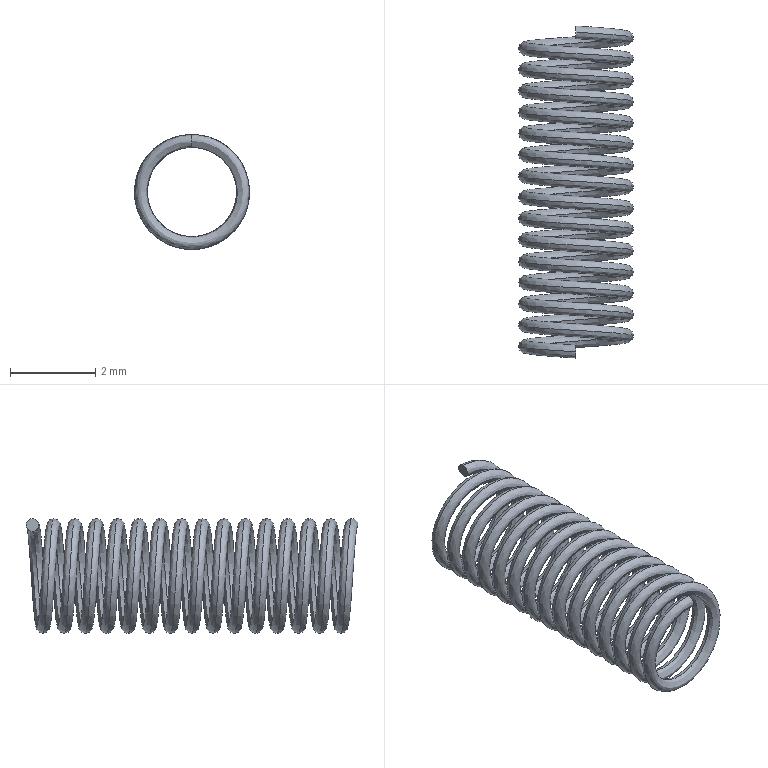Part | SolidWorks | features Helix 1, RefAxis 1, Sweep 1 | 1 solid | 4 faces | box 2.7 x 7.8 x 2.7 mm | volume 7.972 mm3 | spline 2 | plane 2